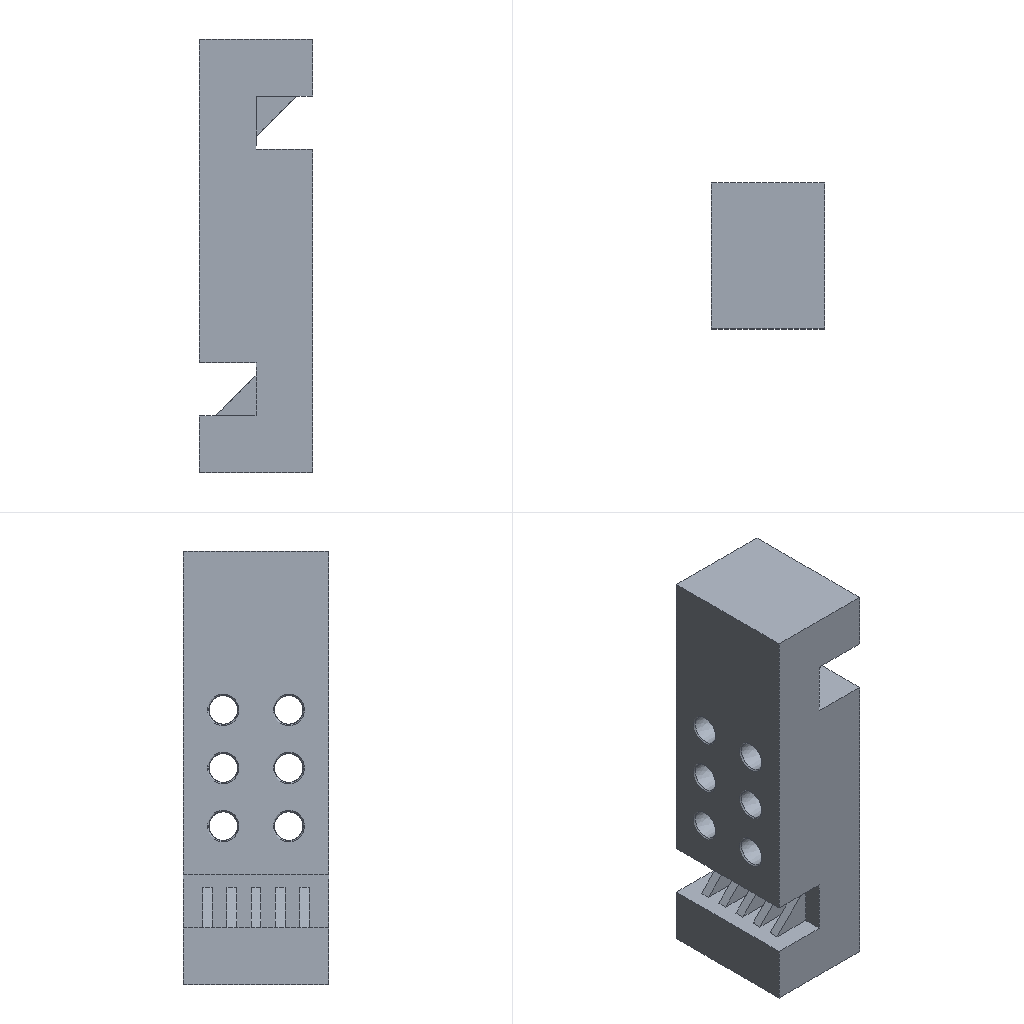Simulation study | ansys workbench
Set-up summary:
category,name,step,type,value,unit,region
solver,ansys_workbench
units,mm-N-s-tonne (MPa),,stated,"/units,MPA"
analysis,LS1,,static
load_step,LS1,LS1,static,nsubst=1; time=1
load_step,LS2,LS2,static,nsubst=1; time=2
mesh,nodes,,,261860
mesh,elements,,,184263
element_type,SOLID187,,,174513
element_type,CONTA174,,,4800
element_type,TARGE170,,,3888
element_type,SURF154,,,1062
material,Structural Steel,,E,200000,tonne s^-2 mm^-1
material,Structural Steel,,nu,0.3
material,Structural Steel,,density,7.85e-09,tonne mm^-3
material,Structural Steel,,conductivity,60.5,tonne mm s^-3 C^-1
material,Structural Steel,,specific_heat,4.34e+08,mm^2 s^-2 C^-1
material,Structural Steel,,cte,1.2e-05,C^-1
material,Structural Steel,,permeability,10000
material,Structural Steel,,resistivity,0.00017,ohm mm
material,mat 29,,E,200000,tonne s^-2 mm^-1
material,mat 29,,nu,0.3
material,mat 29,,density,7.85e-09,tonne mm^-3
material,mat 29,,conductivity,60.5,tonne mm s^-3 C^-1
material,mat 29,,specific_heat,4.34e+08,mm^2 s^-2 C^-1
material,mat 29,,cte,1.2e-05,C^-1
material,mat 29,,permeability,10000
material,mat 29,,resistivity,0.00017,ohm mm
load,Define Force Using Surface Effect Elements,LS1,surface-effect pres face 3,-0.3546,,SURF154 #35
load,,LS1,force,"6000 [dir=(1, 0, 0) n=6]",,node list
bc,Fixed Supports,model,fixed,[dofs=ALL],,_FIXEDSU
bc,,LS2,prescribed ux,table _FIX [dofs=UX n=6],,node list
contact,Frictional - ________|____1 ? ________-0|____1,,standard (frictionless/frictional),friction=0.2; element=CONTA174
contact,contact 2,,bonded (always),element=CONTA174
contact,contact 3,,bonded (always),element=CONTA174
contact,contact 4,,bonded (always),element=CONTA174
contact,contact 5,,bonded (always),element=CONTA174
contact,contact 6,,bonded (always),element=CONTA174
contact,contact 7,,bonded (always),element=CONTA174
contact,contact 8,,bonded (always),element=CONTA174
contact,contact 9,,bonded (always),element=CONTA174
contact,contact 10,,bonded (always),element=CONTA174
contact,contact 11,,bonded (always),element=CONTA174
contact,contact 12,,bonded (always),element=CONTA174
contact,contact 13,,bonded (always),element=CONTA174
named_set,_FIXEDSU,,node,2233
Ansys APDL input file, long lists of numbers shortened:
/batch
/config,noeldb,1     ! force off writing results to database
*get,_wallstrt,active,,time,wall
! ANSYS input file written by Workbench version 2021 R1
! File used for geometry attach:
/title,__--____ (B5)
! ****** Begin Custom Load Command Snippet ******
/COM, ACT Extensions:
/COM,     LSDYNA, 2021.1
/COM,
! ****** End   Custom Load Command Snippet ******
*DIM,_wb_ProjectScratch_dir,string,248
_wb_ProjectScratch_dir(1) = ''
*DIM,_wb_SolverFiles_dir,string,248
_wb_SolverFiles_dir(1) = ''
*DIM,_wb_userfiles_dir,string,248
_wb_userfiles_dir(1) = ''
/com,--- Data in consistent NMM units. See Solving Units in the help system for more information.
/units,MPA
/nopr
/wb,file,start              !  signify a WB generated input file
/prep7
! Turn off shape checking because checks already performed inside WB mesher.
! See help system for more information.
SHPP,OFF,,NOWARN
/nolist
etcon,set             ! allow ANSYS to choose best KEYOP's for 180x elements, resets any applicable keyopt to MAPDL defaults
/com,*********** Nodes for the whole assembly ***********
nblock,3,,288026
(1i9,3e20.9e3)
        1    -2.300000000E+01     1.350000000E+01     5.950000000E+01
! (261841 more lines like these left out)
-1
/com,*********** Nodes for all Remote Points ***********
nblock,3
(1i9,3e20.9e3)
   261843    -2.350000000E+01     1.349999955E+01     6.550000000E+01
! (17 more lines like these left out)
-1
/wb,elem,start            !  set before creation of elements
/com,*********** Elements for Body 1 "________|____1" ***********
et,1,187
eblock,19,solid,,87543
(19i9)
        1        1        1        1        0        0        0        0       10        0    86971   138030   148822   140988   148797   199430   226805   199424   199429
! (175085 more lines like these left out)
-1
/com,*********** Elements for Body 2 "________-0|____1" ***********
et,2,187
eblock,19,solid,,86970
(19i9)
        2        2        2        2        0        0        0        0       10        0        1     2725    18194     3037    18176    37876    40129    37870    37875
! (173939 more lines like these left out)
-1
/wb,elem,end               !  done creating elements
/com,*********** Send User Defined Coordinate System(s) ***********
csys,0
toffst,273.15,  ! Temperature offset from absolute zero
/com,*********** Set Reference Temperature ***********
tref,22.
/wb,mat,start              !  starting to send materials
/com,*********** Send Materials ***********
Temperature = 'TEMP' ! Temperature
MP,DENS,1,7.85e-09,	! tonne mm^-3
MP,ALPX,1,1.2e-05,	! C^-1
MP,C,1,434000000,	! mm^2 s^-2 C^-1
MP,KXX,1,60.5,	! tonne mm s^-3 C^-1
MP,RSVX,1,0.00017,	! ohm mm
MP,EX,1,200000,	! tonne s^-2 mm^-1
MP,NUXY,1,0.3,
MP,MURX,1,10000,
Temperature = 'TEMP' ! Temperature
MP,DENS,2,7.85e-09,	! tonne mm^-3
MP,ALPX,2,1.2e-05,	! C^-1
MP,C,2,434000000,	! mm^2 s^-2 C^-1
MP,KXX,2,60.5,	! tonne mm s^-3 C^-1
MP,RSVX,2,0.00017,	! ohm mm
MP,EX,2,200000,	! tonne s^-2 mm^-1
MP,NUXY,2,0.3,
MP,MURX,2,10000,
/wb,mat,end                !  done sending materials
!************************* Model Summary ********************
!________|____1,	结构钢,	matid,	1
!________-0|____1,	结构钢,	matid,	2
!************************* End Model Summary ********************
! get the diagonal of the bounding box. Needed later for other things
*get,_xmin,node,,mnloc,x
*get,_ymin,node,,mnloc,y
*get,_zmin,node,,mnloc,z
*get,_xmax,node,,mxloc,x
*get,_ymax,node,,mxloc,y
*get,_zmax,node,,mxloc,z
_ASMDIAG=(_xmax-_xmin)*(_xmax-_xmin)+(_ymax-_ymin)*(_ymax-_ymin)+(_zmax-_zmin)*(_zmax-_zmin)
_ASMDIAG=SQRT(_ASMDIAG)
/wb,contact,start          !  starting to send contact
/com,*********** Create Contact "摩擦的 - ________|____1 至 ________-0|____1" ***********
/com,            Real Constant Set For Above Contact Is 4 & 3
*set,tid,4
*set,cid,3
r,tid
r,cid
et,tid,170
et,cid,174
eblock,10,,,1944
(15i9)
   203220        4        4        4        0   132386   132797   132819   132819   162941   165336   132819   162942
! (1943 more lines like these left out)
-1
eblock,10,,,1944
(15i9)
   205164        3        3        3        0   132386   132797   132819   132819   162941   165336   132819   162942
! (1943 more lines like these left out)
-1
eblock,10,,,1944
(15i9)
   207108        3        4        3        0     1859     2270     2292     2292    32210    34579     2292    32211
! (1943 more lines like these left out)
-1
eblock,10,,,1944
(15i9)
   209052        4        3        4        0     1859     2270     2292     2292    32210    34579     2292    32211
! (1943 more lines like these left out)
-1
keyo,cid,8,2               ! auto create asymmetric contact (from Program Controlled setting)
keyo,cid,10,0              ! adjust contact stiffness each NR iteration (from Program Controlled setting)
keyo,cid,12,0              ! standard contact
mp,mu,cid,0.2       ! unitless
keyo,cid,18,1              ! small sliding turned on by application
keyo,cid,2,0               ! augmented Lagrange (from Program Controlled setting)
keyo,cid,4,0               ! on Gauss point (from Program Controlled setting)
keyo,cid,9,0               ! use real geometry with stepped effects
keyo,cid,7,0               ! No Prediction
rmod,tid,3,1.       ! FKN
rmod,tid,5,0.       ! ICONT
rmod,tid,6,0.       ! PINB
rmod,tid,10,0.      ! CNOF
rmod,tid,12,0.      ! FKT
rmod,tid,36,232     ! WB DSID
rmod,cid,3,1.       ! FKN
rmod,cid,5,0.       ! ICONT
rmod,cid,6,0.       ! PINB
rmod,cid,10,0.      ! CNOF
rmod,cid,12,0.      ! FKT
rmod,cid,36,232     ! WB DSID
nsel,all
esel,all
/wb,contact,end            !  done creating contacts
/golist
/wb,load,start             !  starting to send loads
/com,*********** Fixed Supports ***********
CMBLOCK,_FIXEDSU,NODE,     2233
(8i10)
       337       338       339       340       341       342       343       344
! (279 more lines like these left out)
cmsel,s,_FIXEDSU
d,all,all
nsel,all
/com,*********** Create Remote Point "内部远程点" ***********
! -------- Remote Point Used by "循环的 - ________-0|____1 至 ________|____1" --------
*set,tid,6
*set,cid,5
et,cid,174
et,tid,170
keyo,tid,2,1               ! Don't fix the pilot node
keyo,tid,4,111111
keyo,cid,12,5              ! Bonded Contact
keyo,cid,4,1               ! Deformable RBE3 style load
keyo,cid,2,2               ! MPC style contact
eblock,10,,,64
(15i9)
   210996        5        5        5        0       23      605      606      606    18340    22515      606    18341
! (63 more lines like these left out)
-1
*set,_npilot,261843
_npilot128=_npilot
type,tid
mat ,cid
real,cid
tshape,pilo
en,211060,_npilot
tshape
/com,*********** Create Remote Point "内部远程点 2" ***********
! -------- Remote Point Used by "循环的 - ________-0|____1 至 ________|____1" --------
*set,tid,8
*set,cid,7
et,cid,174
et,tid,170
keyo,tid,2,1               ! Don't fix the pilot node
keyo,tid,4,111111
keyo,cid,12,5              ! Bonded Contact
keyo,cid,4,1               ! Deformable RBE3 style load
keyo,cid,2,2               ! MPC style contact
eblock,10,,,88
(15i9)
   211061        7        7        7        0   131097   136497   136481   136481   152835   189100   136481   152834
! (87 more lines like these left out)
-1
*set,_npilot,261844
_npilot129=_npilot
type,tid
mat ,cid
real,cid
tshape,pilo
en,211149,_npilot
tshape
/com,*********** Create Remote Point "内部远程点 3" ***********
! -------- Remote Point Used by "循环的 - ________-0|____1 至 ________|____1" --------
*set,tid,10
*set,cid,9
et,cid,174
et,tid,170
keyo,tid,2,1               ! Don't fix the pilot node
keyo,tid,4,111111
keyo,cid,12,5              ! Bonded Contact
keyo,cid,4,1               ! Deformable RBE3 style load
keyo,cid,2,2               ! MPC style contact
eblock,10,,,64
(15i9)
   211150        9        9        9        0      642     4850      650      650    22824    22889      650    22820
! (63 more lines like these left out)
-1
*set,_npilot,261845
_npilot165=_npilot
type,tid
mat ,cid
real,cid
tshape,pilo
en,211214,_npilot
tshape
/com,*********** Create Remote Point "内部远程点 4" ***********
! -------- Remote Point Used by "循环的 - ________-0|____1 至 ________|____1" --------
*set,tid,12
*set,cid,11
et,cid,174
et,tid,170
keyo,tid,2,1               ! Don't fix the pilot node
keyo,tid,4,111111
keyo,cid,12,5              ! Bonded Contact
keyo,cid,4,1               ! Deformable RBE3 style load
keyo,cid,2,2               ! MPC style contact
eblock,10,,,88
(15i9)
   211215       11       11       11        0   131171   136477   136462   136462   153482   189018   136462   153481
! (87 more lines like these left out)
-1
*set,_npilot,261846
_npilot166=_npilot
type,tid
mat ,cid
real,cid
tshape,pilo
en,211303,_npilot
tshape
/com,*********** Create Remote Point "内部远程点 5" ***********
! -------- Remote Point Used by "循环的 - ________-0|____1 至 ________|____1" --------
*set,tid,14
*set,cid,13
et,cid,174
et,tid,170
keyo,tid,2,1               ! Don't fix the pilot node
keyo,tid,4,111111
keyo,cid,12,5              ! Bonded Contact
keyo,cid,4,1               ! Deformable RBE3 style load
keyo,cid,2,2               ! MPC style contact
eblock,10,,,64
(15i9)
   211304       13       13       13        0      562      587     4858     4858    22155    22369     4858    22159
! (63 more lines like these left out)
-1
*set,_npilot,261847
_npilot170=_npilot
type,tid
mat ,cid
real,cid
tshape,pilo
en,211368,_npilot
tshape
/com,*********** Create Remote Point "内部远程点 6" ***********
! -------- Remote Point Used by "循环的 - ________-0|____1 至 ________|____1" --------
*set,tid,16
*set,cid,15
et,cid,174
et,tid,170
keyo,tid,2,1               ! Don't fix the pilot node
keyo,tid,4,111111
keyo,cid,12,5              ! Bonded Contact
keyo,cid,4,1               ! Deformable RBE3 style load
keyo,cid,2,2               ! MPC style contact
eblock,10,,,88
(15i9)
   211369       15       15       15        0   131126   131127   136445   136445   153087   153100   136445   153091
! (87 more lines like these left out)
-1
*set,_npilot,261848
_npilot171=_npilot
type,tid
mat ,cid
real,cid
tshape,pilo
en,211457,_npilot
tshape
/com,*********** Create Remote Point "内部远程点 7" ***********
! -------- Remote Point Used by "循环的 - ________-0|____1 至 ________|____1" --------
*set,tid,18
*set,cid,17
et,cid,174
et,tid,170
keyo,tid,2,1               ! Don't fix the pilot node
keyo,tid,4,111111
keyo,cid,12,5              ! Bonded Contact
keyo,cid,4,1               ! Deformable RBE3 style load
keyo,cid,2,2               ! MPC style contact
eblock,10,,,64
(15i9)
   211458       17       17       17        0      704      705      717      717    23345    23356      717    23346
! (63 more lines like these left out)
-1
*set,_npilot,261849
_npilot175=_npilot
type,tid
mat ,cid
real,cid
tshape,pilo
en,211522,_npilot
tshape
/com,*********** Create Remote Point "内部远程点 8" ***********
! -------- Remote Point Used by "循环的 - ________-0|____1 至 ________|____1" --------
*set,tid,20
*set,cid,19
et,cid,174
et,tid,170
keyo,tid,2,1               ! Don't fix the pilot node
keyo,tid,4,111111
keyo,cid,12,5              ! Bonded Contact
keyo,cid,4,1               ! Deformable RBE3 style load
keyo,cid,2,2               ! MPC style contact
eblock,10,,,88
(15i9)
   211523       19       19       19        0   130654   131258   136505   136505   149638   154182   136505   149639
! (87 more lines like these left out)
-1
*set,_npilot,261850
_npilot176=_npilot
type,tid
mat ,cid
real,cid
tshape,pilo
en,211611,_npilot
tshape
/com,*********** Create Remote Point "内部远程点 9" ***********
! -------- Remote Point Used by "循环的 - ________-0|____1 至 ________|____1" --------
*set,tid,22
*set,cid,21
et,cid,174
et,tid,170
keyo,tid,2,1               ! Don't fix the pilot node
keyo,tid,4,111111
keyo,cid,12,5              ! Bonded Contact
keyo,cid,4,1               ! Deformable RBE3 style load
keyo,cid,2,2               ! MPC style contact
eblock,10,,,64
(15i9)
   211612       21       21       21        0      553      554      728      728    22080    22093      728    22081
! (63 more lines like these left out)
-1
*set,_npilot,261851
_npilot180=_npilot
type,tid
mat ,cid
real,cid
tshape,pilo
en,211676,_npilot
tshape
/com,*********** Create Remote Point "内部远程点 10" ***********
! -------- Remote Point Used by "循环的 - ________-0|____1 至 ________|____1" --------
*set,tid,24
*set,cid,23
et,cid,174
et,tid,170
keyo,tid,2,1               ! Don't fix the pilot node
keyo,tid,4,111111
keyo,cid,12,5              ! Bonded Contact
keyo,cid,4,1               ! Deformable RBE3 style load
keyo,cid,2,2               ! MPC style contact
eblock,10,,,88
(15i9)
   211677       23       23       23        0   131255   131256   136518   136518   154164   154173   136518   154167
! (87 more lines like these left out)
-1
*set,_npilot,261852
_npilot181=_npilot
type,tid
mat ,cid
real,cid
tshape,pilo
en,211765,_npilot
tshape
/com,*********** Create Remote Point "内部远程点 11" ***********
! -------- Remote Point Used by "循环的 - ________-0|____1 至 ________|____1" --------
*set,tid,26
*set,cid,25
et,cid,174
et,tid,170
keyo,tid,2,1               ! Don't fix the pilot node
keyo,tid,4,111111
keyo,cid,12,5              ! Bonded Contact
keyo,cid,4,1               ! Deformable RBE3 style load
keyo,cid,2,2               ! MPC style contact
eblock,10,,,64
(15i9)
   211766       25       25       25        0      662      663     4861     4861    22979    22993     4861    22984
! (63 more lines like these left out)
-1
*set,_npilot,261853
_npilot185=_npilot
type,tid
mat ,cid
real,cid
tshape,pilo
en,211830,_npilot
tshape
/com,*********** Create Remote Point "内部远程点 12" ***********
! -------- Remote Point Used by "循环的 - ________-0|____1 至 ________|____1" --------
*set,tid,28
*set,cid,27
et,cid,174
et,tid,170
keyo,tid,2,1               ! Don't fix the pilot node
keyo,tid,4,111111
keyo,cid,12,5              ! Bonded Contact
keyo,cid,4,1               ! Deformable RBE3 style load
keyo,cid,2,2               ! MPC style contact
eblock,10,,,88
(15i9)
   211831       27       27       27        0   130548   130549   136538   136538   148952   148959   136538   148953
! (87 more lines like these left out)
-1
*set,_npilot,261854
_npilot186=_npilot
type,tid
mat ,cid
real,cid
tshape,pilo
en,211919,_npilot
tshape
/com,*********** Create Beam Connection "___ - ________-0|____1 _ ________|____1" ***********
/com,            Real Constant Set For Above Beam Connection Is 29
*set,_bid,29
et,_bid,188
mat,_bid
real,_bid
type,_bid
secnum,_bid
en,203196,261843,261844
sectype,29,beam,csolid
secdata,5.
secoffset,cent
Temperature = 'TEMP' ! Temperature
MP,DENS,29,7.85e-09,	! tonne mm^-3
MP,ALPX,29,1.2e-05,	! C^-1
MP,C,29,434000000,	! mm^2 s^-2 C^-1
MP,KXX,29,60.5,	! tonne mm s^-3 C^-1
MP,RSVX,29,0.00017,	! ohm mm
MP,EX,29,200000,	! tonne s^-2 mm^-1
MP,NUXY,29,0.3,
MP,MURX,29,10000,
/com,*********** Create Beam Connection "___ - ________-0|____1 _ ________|____1" ***********
/com,            Real Constant Set For Above Beam Connection Is 30
*set,_bid,30
et,_bid,188
mat,_bid
real,_bid
type,_bid
secnum,_bid
en,203197,261845,261846
sectype,30,beam,csolid
secdata,5.
secoffset,cent
Temperature = 'TEMP' ! Temperature
MP,DENS,30,7.85e-09,	! tonne mm^-3
MP,ALPX,30,1.2e-05,	! C^-1
MP,C,30,434000000,	! mm^2 s^-2 C^-1
MP,KXX,30,60.5,	! tonne mm s^-3 C^-1
MP,RSVX,30,0.00017,	! ohm mm
MP,EX,30,200000,	! tonne s^-2 mm^-1
MP,NUXY,30,0.3,
MP,MURX,30,10000,
/com,*********** Create Beam Connection "___ - ________-0|____1 _ ________|____1" ***********
/com,            Real Constant Set For Above Beam Connection Is 31
*set,_bid,31
et,_bid,188
mat,_bid
real,_bid
type,_bid
secnum,_bid
en,203198,261847,261848
sectype,31,beam,csolid
secdata,5.
secoffset,cent
Temperature = 'TEMP' ! Temperature
MP,DENS,31,7.85e-09,	! tonne mm^-3
MP,ALPX,31,1.2e-05,	! C^-1
MP,C,31,434000000,	! mm^2 s^-2 C^-1
MP,KXX,31,60.5,	! tonne mm s^-3 C^-1
MP,RSVX,31,0.00017,	! ohm mm
MP,EX,31,200000,	! tonne s^-2 mm^-1
MP,NUXY,31,0.3,
MP,MURX,31,10000,
/com,*********** Create Beam Connection "___ - ________-0|____1 _ ________|____1" ***********
/com,            Real Constant Set For Above Beam Connection Is 32
*set,_bid,32
et,_bid,188
mat,_bid
real,_bid
type,_bid
secnum,_bid
en,203199,261849,261850
sectype,32,beam,csolid
secdata,5.
secoffset,cent
Temperature = 'TEMP' ! Temperature
MP,DENS,32,7.85e-09,	! tonne mm^-3
MP,ALPX,32,1.2e-05,	! C^-1
MP,C,32,434000000,	! mm^2 s^-2 C^-1
MP,KXX,32,60.5,	! tonne mm s^-3 C^-1
MP,RSVX,32,0.00017,	! ohm mm
MP,EX,32,200000,	! tonne s^-2 mm^-1
MP,NUXY,32,0.3,
MP,MURX,32,10000,
/com,*********** Create Beam Connection "___ - ________-0|____1 _ ________|____1" ***********
/com,            Real Constant Set For Above Beam Connection Is 33
*set,_bid,33
et,_bid,188
mat,_bid
real,_bid
type,_bid
secnum,_bid
en,203200,261851,261852
sectype,33,beam,csolid
secdata,5.
secoffset,cent
Temperature = 'TEMP' ! Temperature
MP,DENS,33,7.85e-09,	! tonne mm^-3
MP,ALPX,33,1.2e-05,	! C^-1
MP,C,33,434000000,	! mm^2 s^-2 C^-1
MP,KXX,33,60.5,	! tonne mm s^-3 C^-1
MP,RSVX,33,0.00017,	! ohm mm
MP,EX,33,200000,	! tonne s^-2 mm^-1
MP,NUXY,33,0.3,
MP,MURX,33,10000,
/com,*********** Create Beam Connection "___ - ________-0|____1 _ ________|____1" ***********
/com,            Real Constant Set For Above Beam Connection Is 34
*set,_bid,34
et,_bid,188
mat,_bid
real,_bid
type,_bid
secnum,_bid
en,203201,261853,261854
sectype,34,beam,csolid
secdata,5.
secoffset,cent
Temperature = 'TEMP' ! Temperature
MP,DENS,34,7.85e-09,	! tonne mm^-3
MP,ALPX,34,1.2e-05,	! C^-1
MP,C,34,434000000,	! mm^2 s^-2 C^-1
MP,KXX,34,60.5,	! tonne mm s^-3 C^-1
MP,RSVX,34,0.00017,	! ohm mm
MP,EX,34,200000,	! tonne s^-2 mm^-1
MP,NUXY,34,0.3,
MP,MURX,34,10000,
/com,*********** Define Force Using Surface Effect Elements ***********
local,12,0,0.,0.,0.,0.,0.,0.
csys,0
et,35,154
eblock,10,,,1062
(15i9)
   211920       35       35       35       12   136862   137147   137025   137025   191435   192816   137025   191433
! (1061 more lines like these left out)
-1
esel,s,type,,35
keyop,35,2,1                ! Apply load in local coordinate system
keyop,35,7,1                ! Use original area so load is constant in large deformation
esel,all
*DIM,_loadvari135x,TABLE,3,1,1,TIME,
! Time values
_loadvari135x(1,0,1) = 0.
_loadvari135x(2,0,1) = 1.
_loadvari135x(3,0,1) = 2.
! Load values
_loadvari135x(1,1,1) = 0.
_loadvari135x(2,1,1) = 0.
_loadvari135x(3,1,1) = 0.
*DIM,_loadvari135y,TABLE,3,1,1,TIME,
! Time values
_loadvari135y(1,0,1) = 0.
_loadvari135y(2,0,1) = 1.
_loadvari135y(3,0,1) = 2.
! Load values
_loadvari135y(1,1,1) = 0.
_loadvari135y(2,1,1) = 0.
_loadvari135y(3,1,1) = 0.
*DIM,_loadvari135z,TABLE,3,1,1,TIME,
! Time values
_loadvari135z(1,0,1) = 0.
_loadvari135z(2,0,1) = 1.
_loadvari135z(3,0,1) = 2.
! Load values
_loadvari135z(1,1,1) = 0.
_loadvari135z(2,1,1) = 0.
_loadvari135z(3,1,1) = -0.3546
/com,*********** Create Bolt Pretension "_____" ***********
*set,_pretnode,261855
_nbolt125 = 261855               ! that will be the pretension node number
*set,_beame1,203196
*set,_beamn1,261843
*set,_beamn2,261844
_centx = .5*(NX(_beamn1)+NX(_beamn2))
_centy = .5*(NY(_beamn1)+NY(_beamn2))
! (8 more lines like these left out)
local,11,0,_centx,_centy,_centz
nmod,_pretnode,0,0,0,,,,1              ! move pretension node to bolt center, don't update centroid
*get,_nmax,ndmx
_center1=_nmax+1
_center2=_nmax+2
n,_center1,
n,_center2,
*get,_bid,elem,_beame1,ATTR,MAT        ! get the material number of beam connection element
mat,_bid
real,_bid
type,_bid
secnum,_bid
emod,_beame1,2,_center1                ! modify the original beam element to half length
e,_center2,_beamn2                     ! create new beam element to span second half of length
*set,_tid,36
et,_tid,179
type,_tid
real,_tid
mat,_tid
secnum,_tid
e,_center1,_center2,_pretnode          ! directly create pretension element
SECTYPE,_tid,PRETENSION
secdata,_pretnode,_dirx,_diry,_dirz    ! pretension directon set from the 2 beam connection nodes
csys,0
/com,*********** Create Bolt Pretension "_____ 2" ***********
*set,_pretnode,261856
_nbolt196 = 261856               ! that will be the pretension node number
*set,_beame1,203197
*set,_beamn1,261845
*set,_beamn2,261846
_centx = .5*(NX(_beamn1)+NX(_beamn2))
_centy = .5*(NY(_beamn1)+NY(_beamn2))
! (8 more lines like these left out)
local,11,0,_centx,_centy,_centz
nmod,_pretnode,0,0,0,,,,1              ! move pretension node to bolt center, don't update centroid
*get,_nmax,ndmx
_center1=_nmax+1
_center2=_nmax+2
n,_center1,
n,_center2,
*get,_bid,elem,_beame1,ATTR,MAT        ! get the material number of beam connection element
mat,_bid
real,_bid
type,_bid
secnum,_bid
emod,_beame1,2,_center1                ! modify the original beam element to half length
e,_center2,_beamn2                     ! create new beam element to span second half of length
*set,_tid,37
et,_tid,179
type,_tid
real,_tid
mat,_tid
secnum,_tid
e,_center1,_center2,_pretnode          ! directly create pretension element
SECTYPE,_tid,PRETENSION
secdata,_pretnode,_dirx,_diry,_dirz    ! pretension directon set from the 2 beam connection nodes
csys,0
/com,*********** Create Bolt Pretension "_____ 3" ***********
*set,_pretnode,261857
_nbolt197 = 261857               ! that will be the pretension node number
*set,_beame1,203198
*set,_beamn1,261847
*set,_beamn2,261848
_centx = .5*(NX(_beamn1)+NX(_beamn2))
_centy = .5*(NY(_beamn1)+NY(_beamn2))
! (8 more lines like these left out)
local,11,0,_centx,_centy,_centz
nmod,_pretnode,0,0,0,,,,1              ! move pretension node to bolt center, don't update centroid
*get,_nmax,ndmx
_center1=_nmax+1
_center2=_nmax+2
n,_center1,
n,_center2,
*get,_bid,elem,_beame1,ATTR,MAT        ! get the material number of beam connection element
mat,_bid
real,_bid
type,_bid
secnum,_bid
emod,_beame1,2,_center1                ! modify the original beam element to half length
e,_center2,_beamn2                     ! create new beam element to span second half of length
*set,_tid,38
et,_tid,179
type,_tid
real,_tid
mat,_tid
secnum,_tid
e,_center1,_center2,_pretnode          ! directly create pretension element
SECTYPE,_tid,PRETENSION
secdata,_pretnode,_dirx,_diry,_dirz    ! pretension directon set from the 2 beam connection nodes
csys,0
/com,*********** Create Bolt Pretension "_____ 4" ***********
*set,_pretnode,261858
_nbolt198 = 261858               ! that will be the pretension node number
*set,_beame1,203199
*set,_beamn1,261849
*set,_beamn2,261850
_centx = .5*(NX(_beamn1)+NX(_beamn2))
_centy = .5*(NY(_beamn1)+NY(_beamn2))
! (8 more lines like these left out)
local,11,0,_centx,_centy,_centz
nmod,_pretnode,0,0,0,,,,1              ! move pretension node to bolt center, don't update centroid
*get,_nmax,ndmx
_center1=_nmax+1
_center2=_nmax+2
n,_center1,
n,_center2,
*get,_bid,elem,_beame1,ATTR,MAT        ! get the material number of beam connection element
mat,_bid
real,_bid
type,_bid
secnum,_bid
emod,_beame1,2,_center1                ! modify the original beam element to half length
e,_center2,_beamn2                     ! create new beam element to span second half of length
*set,_tid,39
et,_tid,179
type,_tid
real,_tid
mat,_tid
secnum,_tid
e,_center1,_center2,_pretnode          ! directly create pretension element
SECTYPE,_tid,PRETENSION
secdata,_pretnode,_dirx,_diry,_dirz    ! pretension directon set from the 2 beam connection nodes
csys,0
/com,*********** Create Bolt Pretension "_____ 5" ***********
*set,_pretnode,261859
_nbolt199 = 261859               ! that will be the pretension node number
*set,_beame1,203200
*set,_beamn1,261851
*set,_beamn2,261852
_centx = .5*(NX(_beamn1)+NX(_beamn2))
_centy = .5*(NY(_beamn1)+NY(_beamn2))
! (8 more lines like these left out)
local,11,0,_centx,_centy,_centz
nmod,_pretnode,0,0,0,,,,1              ! move pretension node to bolt center, don't update centroid
*get,_nmax,ndmx
_center1=_nmax+1
_center2=_nmax+2
n,_center1,
n,_center2,
*get,_bid,elem,_beame1,ATTR,MAT        ! get the material number of beam connection element
mat,_bid
real,_bid
type,_bid
secnum,_bid
emod,_beame1,2,_center1                ! modify the original beam element to half length
e,_center2,_beamn2                     ! create new beam element to span second half of length
*set,_tid,40
et,_tid,179
type,_tid
real,_tid
mat,_tid
secnum,_tid
e,_center1,_center2,_pretnode          ! directly create pretension element
SECTYPE,_tid,PRETENSION
secdata,_pretnode,_dirx,_diry,_dirz    ! pretension directon set from the 2 beam connection nodes
csys,0
/com,*********** Create Bolt Pretension "_____ 6" ***********
*set,_pretnode,261860
_nbolt200 = 261860               ! that will be the pretension node number
*set,_beame1,203201
*set,_beamn1,261853
*set,_beamn2,261854
_centx = .5*(NX(_beamn1)+NX(_beamn2))
_centy = .5*(NY(_beamn1)+NY(_beamn2))
! (8 more lines like these left out)
local,11,0,_centx,_centy,_centz
nmod,_pretnode,0,0,0,,,,1              ! move pretension node to bolt center, don't update centroid
*get,_nmax,ndmx
_center1=_nmax+1
_center2=_nmax+2
n,_center1,
n,_center2,
*get,_bid,elem,_beame1,ATTR,MAT        ! get the material number of beam connection element
mat,_bid
real,_bid
type,_bid
secnum,_bid
emod,_beame1,2,_center1                ! modify the original beam element to half length
e,_center2,_beamn2                     ! create new beam element to span second half of length
*set,_tid,41
et,_tid,179
type,_tid
real,_tid
mat,_tid
secnum,_tid
e,_center1,_center2,_pretnode          ! directly create pretension element
SECTYPE,_tid,PRETENSION
secdata,_pretnode,_dirx,_diry,_dirz    ! pretension directon set from the 2 beam connection nodes
csys,0
/gst,on,on
fini
*get,_numnode,node,0,count
*get,_numelem,elem,0,count
*get, _MAXELEMNUM, elem, 0, NUM, MAX
*get, _MAXNODENUM, node, 0, NUM, MAX
*get, _MAXELEMTYPE, etyp, 0, NUM, MAX
*get, _MAXREALCONST, real, 0, NUM, MAX
/go
/wb,load,end               !  done creating loads
/com,--- Number of total nodes = %_numnode%
/com,--- Number of contact elements = 9750
/com,--- Number of spring elements = 0
/com,--- Number of bearing elements = 0
/com,--- Number of solid elements = 174513
/com,--- Number of condensed parts = 0
/com,--- Number of total elements = %_numelem%
*get,_wallbsol,active,,time,wall
/com,****************************************************************************
/com,*************************    SOLUTION       ********************************
/com,****************************************************************************
/solu
antype,0                   ! static analysis
_thickRatio=  1     ! Ratio of thick parts in the model
eqsl,pcg,1e-8,,,,,,1
cntr,print,1               ! print out contact info and also make no initial contact an error
dmpoption,emat,no             ! Don't combine emat file for DANSYS
dmpoption,esav,no             ! Don't combine esav file for DANSYS
nldiag,cont,iter           ! print out contact info each equilibrium iteration
rescontrol,define,last,last,,dele	   ! Program Controlled
/com,****************************************************
/com,******************* SOLVE FOR LS 1 OF 2 ****************
esel,s,type,,35
nsle
sfe,all,1,pres,1,%_loadvari135x%
sfe,all,2,pres,1,%_loadvari135y%
sfe,all,3,pres,1,%_loadvari135z%
nsel,all
esel,all
/nopr
/gopr
/nolist
f,261855,fx,1000.
f,261856,fx,1000.
f,261857,fx,1000.
f,261858,fx,1000.
f,261859,fx,1000.
f,261860,fx,1000.
autots,on                  ! Workbench Program Controlled automatic time stepping
nsub,1,10,1                ! due to presence of general nonlinear
time,1.
outres,erase
outres,all,none
outres,nsol,all,
outres,rsol,all
outres,eangl,all
outres,etmp,all
outres,veng,all
outres,strs,all,
outres,epel,all,
outres,eppl,all,
outres,cont,all,
/nopr
esel,s,type,,29
esel,a,type,,30,34
cm,_elmisc,elem
esel,all
/gopr
outres,misc,all,_elmisc
! *********** WB SOLVE COMMAND ***********
! check interactive state
*get,ANSINTER_,active,,int
*if,ANSINTER_,ne,0,then
/eof
*endif
solve
/com *************** Write FE CONNECTORS *********
CEWRITE,file,ce,,INTE
/com,****************************************************
/com,*************** FINISHED SOLVE FOR LS 1 *************
/com,****************************************************
/com,******************* SOLVE FOR LS 2 OF 2 ****************
/nopr
/gopr
/nolist
fdel,261855,all
d,261855,ux,%_FIX%
fdel,261856,all
d,261856,ux,%_FIX%
fdel,261857,all
d,261857,ux,%_FIX%
fdel,261858,all
d,261858,ux,%_FIX%
fdel,261859,all
d,261859,ux,%_FIX%
fdel,261860,all
d,261860,ux,%_FIX%
autots,on                  ! Workbench Program Controlled automatic time stepping
nsub,1,10,1                ! due to presence of general nonlinear
time,2.
outres,erase
outres,all,none
outres,nsol,all,
outres,rsol,all
outres,eangl,all
outres,etmp,all
outres,veng,all
outres,strs,all,
outres,epel,all,
outres,eppl,all,
outres,cont,all,
outres,misc,all,_elmisc
solve
/com,****************************************************
/com,*************** FINISHED SOLVE FOR LS 2 *************
*get,_wallasol,active,,time,wall
/nopr
*get,_numnode,node,0,count
*get,_numelem,elem,0,count
*get, _MAXELEMNUM, elem, 0, NUM, MAX
*get, _MAXNODENUM, node, 0, NUM, MAX,,,INTERNAL
*get, _MAXELEMTYPE, etyp, 0, NUM, MAX
*get, _MAXREALCONST, real, 0, NUM, MAX
/gopr
*get,_PCGITER,active,,solu,cgiter
/post1
xmlo,ENCODING,ISO-8859-1
xmlo,parm
/xml,parm,xml
fini
/gopr
*get,_walldone,active,,time,wall
_preptime=(_wallbsol-_wallstrt)*3600
_solvtime=(_wallasol-_wallbsol)*3600
_posttime=(_walldone-_wallasol)*3600
_totaltim=(_walldone-_wallstrt)*3600
*get,_dlbratio,active,0,solu,dlbr
*get,_combtime,active,0,solu,comb
/com,--- Total number of nodes = %_numnode%
/com,--- Total number of elements = %_numelem%
/com,--- Element load balance ratio = %_dlbratio%
/com,--- Time to combine distributed files = %_combtime%
/wb,file,end               ! done with WB generated input
Results summary:
result,analyses[0].index,,,1
result,analyses[0].system,,,SYS-1
result,analyses[0].deck,,,deck.dat
result,analyses[0].solve_status,,,completed
result,analyses[0].analysis_type,,,static
result,analyses[0].physics,,,mechanical
result,analyses[0].unit_system,,,"NMM: mm, ton, N, s, mV, mA, degC"
result,analyses[0].n_sets,,,2
result,analyses[0].load_steps[0].set,set=1,,1
result,analyses[0].load_steps[0].time_or_freq,set=1,,1
result,analyses[0].load_steps[0].max_displacement_magnitude,set=1,,0.00366
result,analyses[0].load_steps[0].max_von_mises_nodal,set=1,,7.786
result,analyses[0].load_steps[0].reaction_force_sum_xyz[1],set=1,,7.6533e-07
result,analyses[0].load_steps[0].reaction_force_sum_xyz[2],set=1,,3.86769e-09
result,analyses[0].load_steps[0].reaction_force_sum_xyz[3],set=1,,3.0966e-09
result,analyses[0].load_steps[1].set,set=2,,2
result,analyses[0].load_steps[1].time_or_freq,set=2,,2
result,analyses[0].load_steps[1].max_displacement_magnitude,set=2,,0.005171
result,analyses[0].load_steps[1].max_von_mises_nodal,set=2,,7.892
result,analyses[0].load_steps[1].reaction_force_sum_xyz[1],set=2,,5926.04
result,analyses[0].load_steps[1].reaction_force_sum_xyz[2],set=2,,-3.56583e-11
result,analyses[0].load_steps[1].reaction_force_sum_xyz[3],set=2,,1000
result,geometry_export[0][0],,,.step
result,geometry_export[0][1],,,ok
result,geometry_export[0][2],,,2